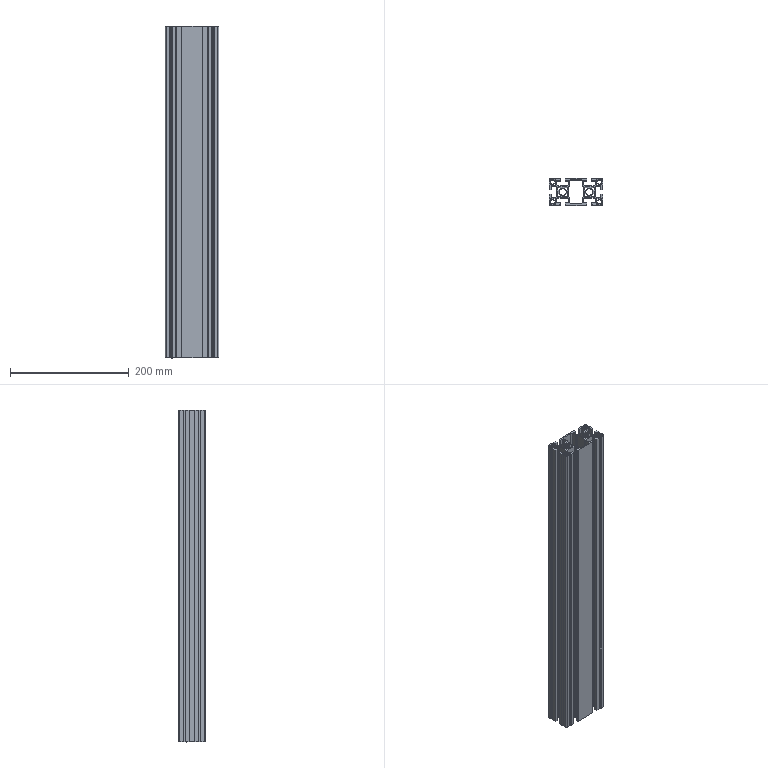Part | STEP file | 4590-705 Al 3 (front col) | 1 solid | 366 faces | box 90 x 45 x 558 mm | volume 654369 mm3 | plane 254 | cylinder 112 | commonest cylinder face diameters 2 x64 8 x20 12 x16 4 x12